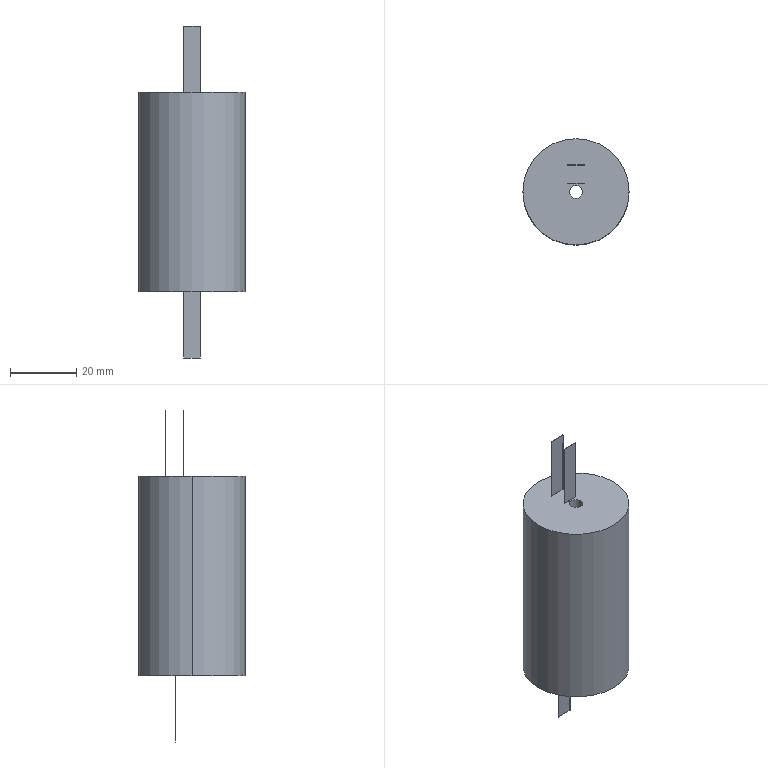Part | SolidWorks | features ICE 2, Extrusion 1 | 1 solid | 21 faces | box 32 x 32 x 100 mm | volume 47531 mm3 | plane 17 | cylinder 4 | commonest cylinder face diameters 4 x2 32 x2
STEP:
#1=CARTESIAN_POINT('',(-2.,0.,60.));
#2=VERTEX_POINT('',#1);
#3=CARTESIAN_POINT('',(2.,0.,60.));
#4=VERTEX_POINT('',#3);
#5=CARTESIAN_POINT('',(0.,0.,60.));
#6=DIRECTION('',(0.,0.,1.));
#7=DIRECTION('',(1.,0.,0.));
#8=AXIS2_PLACEMENT_3D('',#5,#6,#7);
#9=CIRCLE('',#8,2.);
#10=EDGE_CURVE('',#2,#4,#9,.T.);
#11=ORIENTED_EDGE('',*,*,#10,.T.);
#12=CARTESIAN_POINT('',(2.,0.,0.));
#13=VERTEX_POINT('',#12);
#14=CARTESIAN_POINT('',(2.,0.,60.));
#15=DIRECTION('',(0.,0.,-1.));
#16=VECTOR('',#15,1000.);
#17=LINE('',#14,#16);
#18=EDGE_CURVE('',#4,#13,#17,.T.);
#19=ORIENTED_EDGE('',*,*,#18,.T.);
#20=CARTESIAN_POINT('',(-2.,0.,0.));
#21=VERTEX_POINT('',#20);
#22=CARTESIAN_POINT('',(0.,0.,0.));
#23=DIRECTION('',(0.,0.,1.));
#24=DIRECTION('',(1.,0.,0.));
#25=AXIS2_PLACEMENT_3D('',#22,#23,#24);
#26=CIRCLE('',#25,2.);
#27=EDGE_CURVE('',#21,#13,#26,.T.);
#28=ORIENTED_EDGE('',*,*,#27,.F.);
#29=CARTESIAN_POINT('',(-2.,0.,60.));
#30=DIRECTION('',(0.,0.,-1.));
#31=VECTOR('',#30,1000.);
#32=LINE('',#29,#31);
#33=EDGE_CURVE('',#2,#21,#32,.T.);
#34=ORIENTED_EDGE('',*,*,#33,.F.);
#35=EDGE_LOOP('',(#11,#19,#28,#34));
#36=FACE_OUTER_BOUND('',#35,.T.);
#37=CARTESIAN_POINT('',(0.,0.,60.));
#38=DIRECTION('',(0.,0.,-1.));
#39=DIRECTION('',(-1.,0.,0.));
#40=AXIS2_PLACEMENT_3D('',#37,#38,#39);
#41=CYLINDRICAL_SURFACE('',#40,2.);
#42=ADVANCED_FACE('',(#36),#41,.F.);
#43=CARTESIAN_POINT('',(16.,0.,60.));
#44=VERTEX_POINT('',#43);
#45=CARTESIAN_POINT('',(-16.,0.,60.));
#46=VERTEX_POINT('',#45);
#47=CARTESIAN_POINT('',(0.,0.,60.));
#48=DIRECTION('',(0.,0.,1.));
#49=DIRECTION('',(1.,0.,0.));
#50=AXIS2_PLACEMENT_3D('',#47,#48,#49);
#51=CIRCLE('',#50,16.);
#52=EDGE_CURVE('',#44,#46,#51,.T.);
#53=ORIENTED_EDGE('',*,*,#52,.F.);
#54=CARTESIAN_POINT('',(16.,0.,0.));
#55=VERTEX_POINT('',#54);
#56=CARTESIAN_POINT('',(16.,0.,60.));
#57=DIRECTION('',(0.,0.,-1.));
#58=VECTOR('',#57,1000.);
#59=LINE('',#56,#58);
#60=EDGE_CURVE('',#44,#55,#59,.T.);
#61=ORIENTED_EDGE('',*,*,#60,.T.);
#62=CARTESIAN_POINT('',(-16.,0.,0.));
#63=VERTEX_POINT('',#62);
#64=CARTESIAN_POINT('',(0.,0.,0.));
#65=DIRECTION('',(0.,0.,1.));
#66=DIRECTION('',(1.,0.,0.));
#67=AXIS2_PLACEMENT_3D('',#64,#65,#66);
#68=CIRCLE('',#67,16.);
#69=EDGE_CURVE('',#55,#63,#68,.T.);
#70=ORIENTED_EDGE('',*,*,#69,.T.);
#71=CARTESIAN_POINT('',(-16.,0.,60.));
#72=DIRECTION('',(0.,0.,-1.));
#73=VECTOR('',#72,1000.);
#74=LINE('',#71,#73);
#75=EDGE_CURVE('',#46,#63,#74,.T.);
#76=ORIENTED_EDGE('',*,*,#75,.F.);
#77=EDGE_LOOP('',(#53,#61,#70,#76));
#78=FACE_OUTER_BOUND('',#77,.T.);
#79=CARTESIAN_POINT('',(0.,0.,60.));
#80=DIRECTION('',(0.,0.,-1.));
#81=DIRECTION('',(-1.,0.,0.));
#82=AXIS2_PLACEMENT_3D('',#79,#80,#81);
#83=CYLINDRICAL_SURFACE('',#82,16.);
#84=ADVANCED_FACE('',(#78),#83,.T.);
#85=CARTESIAN_POINT('',(2.5,8.1,60.));
#86=VERTEX_POINT('',#85);
#87=CARTESIAN_POINT('',(-2.5,8.1,60.));
#88=VERTEX_POINT('',#87);
#89=CARTESIAN_POINT('',(-2.5,8.1,60.));
#90=DIRECTION('',(-1.,0.,0.));
#91=VECTOR('',#90,1000.);
#92=LINE('',#89,#91);
#93=EDGE_CURVE('',#86,#88,#92,.T.);
#94=ORIENTED_EDGE('',*,*,#93,.F.);
#95=CARTESIAN_POINT('',(2.5,8.,60.));
#96=VERTEX_POINT('',#95);
#97=CARTESIAN_POINT('',(2.5,8.1,60.));
#98=DIRECTION('',(0.,1.,0.));
#99=VECTOR('',#98,1000.);
#100=LINE('',#97,#99);
#101=EDGE_CURVE('',#96,#86,#100,.T.);
#102=ORIENTED_EDGE('',*,*,#101,.F.);
#103=CARTESIAN_POINT('',(-2.5,8.,60.));
#104=VERTEX_POINT('',#103);
#105=CARTESIAN_POINT('',(-2.5,8.,60.));
#106=DIRECTION('',(1.,0.,0.));
#107=VECTOR('',#106,1000.);
#108=LINE('',#105,#107);
#109=EDGE_CURVE('',#104,#96,#108,.T.);
#110=ORIENTED_EDGE('',*,*,#109,.F.);
#111=CARTESIAN_POINT('',(-2.5,8.1,60.));
#112=DIRECTION('',(0.,-1.,0.));
#113=VECTOR('',#112,1000.);
#114=LINE('',#111,#113);
#115=EDGE_CURVE('',#88,#104,#114,.T.);
#116=ORIENTED_EDGE('',*,*,#115,.F.);
#117=EDGE_LOOP('',(#94,#102,#110,#116));
#118=FACE_BOUND('',#117,.T.);
#119=CARTESIAN_POINT('',(0.,0.,60.));
#120=DIRECTION('',(0.,0.,1.));
#121=DIRECTION('',(1.,0.,0.));
#122=AXIS2_PLACEMENT_3D('',#119,#120,#121);
#123=CIRCLE('',#122,16.);
#124=EDGE_CURVE('',#46,#44,#123,.T.);
#125=ORIENTED_EDGE('',*,*,#124,.T.);
#126=ORIENTED_EDGE('',*,*,#52,.T.);
#127=EDGE_LOOP('',(#125,#126));
#128=FACE_OUTER_BOUND('',#127,.T.);
#129=ORIENTED_EDGE('',*,*,#10,.F.);
#130=CARTESIAN_POINT('',(0.,0.,60.));
#131=DIRECTION('',(0.,0.,1.));
#132=DIRECTION('',(1.,0.,0.));
#133=AXIS2_PLACEMENT_3D('',#130,#131,#132);
#134=CIRCLE('',#133,2.);
#135=EDGE_CURVE('',#4,#2,#134,.T.);
#136=ORIENTED_EDGE('',*,*,#135,.F.);
#137=EDGE_LOOP('',(#129,#136));
#138=FACE_BOUND('',#137,.T.);
#139=CARTESIAN_POINT('',(-2.5,2.5,60.));
#140=VERTEX_POINT('',#139);
#141=CARTESIAN_POINT('',(2.5,2.5,60.));
#142=VERTEX_POINT('',#141);
#143=CARTESIAN_POINT('',(-2.5,2.5,60.));
#144=DIRECTION('',(1.,0.,0.));
#145=VECTOR('',#144,1000.);
#146=LINE('',#143,#145);
#147=EDGE_CURVE('',#140,#142,#146,.T.);
#148=ORIENTED_EDGE('',*,*,#147,.F.);
#149=CARTESIAN_POINT('',(-2.5,2.6,60.));
#150=VERTEX_POINT('',#149);
#151=CARTESIAN_POINT('',(-2.5,2.6,60.));
#152=DIRECTION('',(0.,-1.,0.));
#153=VECTOR('',#152,1000.);
#154=LINE('',#151,#153);
#155=EDGE_CURVE('',#150,#140,#154,.T.);
#156=ORIENTED_EDGE('',*,*,#155,.F.);
#157=CARTESIAN_POINT('',(2.5,2.6,60.));
#158=VERTEX_POINT('',#157);
#159=CARTESIAN_POINT('',(-2.5,2.6,60.));
#160=DIRECTION('',(-1.,0.,0.));
#161=VECTOR('',#160,1000.);
#162=LINE('',#159,#161);
#163=EDGE_CURVE('',#158,#150,#162,.T.);
#164=ORIENTED_EDGE('',*,*,#163,.F.);
#165=CARTESIAN_POINT('',(2.5,2.6,60.));
#166=DIRECTION('',(0.,1.,0.));
#167=VECTOR('',#166,1000.);
#168=LINE('',#165,#167);
#169=EDGE_CURVE('',#142,#158,#168,.T.);
#170=ORIENTED_EDGE('',*,*,#169,.F.);
#171=EDGE_LOOP('',(#148,#156,#164,#170));
#172=FACE_BOUND('',#171,.T.);
#173=CARTESIAN_POINT('',(0.,0.,60.));
#174=DIRECTION('',(0.,0.,1.));
#175=DIRECTION('',(1.,0.,0.));
#176=AXIS2_PLACEMENT_3D('',#173,#174,#175);
#177=PLANE('',#176);
#178=ADVANCED_FACE('',(#118,#128,#138,#172),#177,.T.);
#179=ORIENTED_EDGE('',*,*,#27,.T.);
#180=CARTESIAN_POINT('',(0.,0.,0.));
#181=DIRECTION('',(0.,0.,1.));
#182=DIRECTION('',(1.,0.,0.));
#183=AXIS2_PLACEMENT_3D('',#180,#181,#182);
#184=CIRCLE('',#183,2.);
#185=EDGE_CURVE('',#13,#21,#184,.T.);
#186=ORIENTED_EDGE('',*,*,#185,.T.);
#187=EDGE_LOOP('',(#179,#186));
#188=FACE_BOUND('',#187,.T.);
#189=CARTESIAN_POINT('',(0.,0.,0.));
#190=DIRECTION('',(0.,0.,1.));
#191=DIRECTION('',(1.,0.,0.));
#192=AXIS2_PLACEMENT_3D('',#189,#190,#191);
#193=CIRCLE('',#192,16.);
#194=EDGE_CURVE('',#63,#55,#193,.T.);
#195=ORIENTED_EDGE('',*,*,#194,.F.);
#196=ORIENTED_EDGE('',*,*,#69,.F.);
#197=EDGE_LOOP('',(#195,#196));
#198=FACE_OUTER_BOUND('',#197,.T.);
#199=CARTESIAN_POINT('',(-2.5,5.,0.));
#200=VERTEX_POINT('',#199);
#201=CARTESIAN_POINT('',(-2.5,5.1,0.));
#202=VERTEX_POINT('',#201);
#203=CARTESIAN_POINT('',(-2.5,5.1,0.));
#204=DIRECTION('',(0.,1.,0.));
#205=VECTOR('',#204,1000.);
#206=LINE('',#203,#205);
#207=EDGE_CURVE('',#200,#202,#206,.T.);
#208=ORIENTED_EDGE('',*,*,#207,.F.);
#209=CARTESIAN_POINT('',(2.5,5.,0.));
#210=VERTEX_POINT('',#209);
#211=CARTESIAN_POINT('',(2.5,5.,0.));
#212=DIRECTION('',(-1.,0.,0.));
#213=VECTOR('',#212,1000.);
#214=LINE('',#211,#213);
#215=EDGE_CURVE('',#210,#200,#214,.T.);
#216=ORIENTED_EDGE('',*,*,#215,.F.);
#217=CARTESIAN_POINT('',(2.5,5.1,0.));
#218=VERTEX_POINT('',#217);
#219=CARTESIAN_POINT('',(2.5,5.1,0.));
#220=DIRECTION('',(0.,-1.,0.));
#221=VECTOR('',#220,1000.);
#222=LINE('',#219,#221);
#223=EDGE_CURVE('',#218,#210,#222,.T.);
#224=ORIENTED_EDGE('',*,*,#223,.F.);
#225=CARTESIAN_POINT('',(2.5,5.1,0.));
#226=DIRECTION('',(1.,0.,0.));
#227=VECTOR('',#226,1000.);
#228=LINE('',#225,#227);
#229=EDGE_CURVE('',#202,#218,#228,.T.);
#230=ORIENTED_EDGE('',*,*,#229,.F.);
#231=EDGE_LOOP('',(#208,#216,#224,#230));
#232=FACE_BOUND('',#231,.T.);
#233=CARTESIAN_POINT('',(0.,0.,0.));
#234=DIRECTION('',(0.,0.,1.));
#235=DIRECTION('',(1.,0.,0.));
#236=AXIS2_PLACEMENT_3D('',#233,#234,#235);
#237=PLANE('',#236);
#238=ADVANCED_FACE('',(#188,#198,#232),#237,.F.);
#239=ORIENTED_EDGE('',*,*,#60,.F.);
#240=ORIENTED_EDGE('',*,*,#124,.F.);
#241=ORIENTED_EDGE('',*,*,#75,.T.);
#242=ORIENTED_EDGE('',*,*,#194,.T.);
#243=EDGE_LOOP('',(#239,#240,#241,#242));
#244=FACE_OUTER_BOUND('',#243,.T.);
#245=CARTESIAN_POINT('',(0.,0.,60.));
#246=DIRECTION('',(0.,0.,-1.));
#247=DIRECTION('',(-1.,0.,0.));
#248=AXIS2_PLACEMENT_3D('',#245,#246,#247);
#249=CYLINDRICAL_SURFACE('',#248,16.);
#250=ADVANCED_FACE('',(#244),#249,.T.);
#251=ORIENTED_EDGE('',*,*,#18,.F.);
#252=ORIENTED_EDGE('',*,*,#135,.T.);
#253=ORIENTED_EDGE('',*,*,#33,.T.);
#254=ORIENTED_EDGE('',*,*,#185,.F.);
#255=EDGE_LOOP('',(#251,#252,#253,#254));
#256=FACE_OUTER_BOUND('',#255,.T.);
#257=CARTESIAN_POINT('',(0.,0.,60.));
#258=DIRECTION('',(0.,0.,-1.));
#259=DIRECTION('',(-1.,0.,0.));
#260=AXIS2_PLACEMENT_3D('',#257,#258,#259);
#261=CYLINDRICAL_SURFACE('',#260,2.);
#262=ADVANCED_FACE('',(#256),#261,.F.);
#263=ORIENTED_EDGE('',*,*,#207,.T.);
#264=CARTESIAN_POINT('',(-2.5,5.1,-20.));
#265=VERTEX_POINT('',#264);
#266=CARTESIAN_POINT('',(-2.5,5.1,-20.));
#267=DIRECTION('',(0.,0.,1.));
#268=VECTOR('',#267,1000.);
#269=LINE('',#266,#268);
#270=EDGE_CURVE('',#265,#202,#269,.T.);
#271=ORIENTED_EDGE('',*,*,#270,.F.);
#272=CARTESIAN_POINT('',(-2.5,5.,-20.));
#273=VERTEX_POINT('',#272);
#274=CARTESIAN_POINT('',(-2.5,5.1,-20.));
#275=DIRECTION('',(0.,1.,0.));
#276=VECTOR('',#275,1000.);
#277=LINE('',#274,#276);
#278=EDGE_CURVE('',#273,#265,#277,.T.);
#279=ORIENTED_EDGE('',*,*,#278,.F.);
#280=CARTESIAN_POINT('',(-2.5,5.,-20.));
#281=DIRECTION('',(0.,0.,1.));
#282=VECTOR('',#281,1000.);
#283=LINE('',#280,#282);
#284=EDGE_CURVE('',#273,#200,#283,.T.);
#285=ORIENTED_EDGE('',*,*,#284,.T.);
#286=EDGE_LOOP('',(#263,#271,#279,#285));
#287=FACE_OUTER_BOUND('',#286,.T.);
#288=CARTESIAN_POINT('',(-2.5,5.1,-20.));
#289=DIRECTION('',(1.,0.,0.));
#290=DIRECTION('',(0.,0.,-1.));
#291=AXIS2_PLACEMENT_3D('',#288,#289,#290);
#292=PLANE('',#291);
#293=ADVANCED_FACE('',(#287),#292,.F.);
#294=ORIENTED_EDGE('',*,*,#229,.T.);
#295=CARTESIAN_POINT('',(2.5,5.1,-20.));
#296=VERTEX_POINT('',#295);
#297=CARTESIAN_POINT('',(2.5,5.1,-20.));
#298=DIRECTION('',(0.,0.,1.));
#299=VECTOR('',#298,1000.);
#300=LINE('',#297,#299);
#301=EDGE_CURVE('',#296,#218,#300,.T.);
#302=ORIENTED_EDGE('',*,*,#301,.F.);
#303=CARTESIAN_POINT('',(2.5,5.1,-20.));
#304=DIRECTION('',(1.,0.,0.));
#305=VECTOR('',#304,1000.);
#306=LINE('',#303,#305);
#307=EDGE_CURVE('',#265,#296,#306,.T.);
#308=ORIENTED_EDGE('',*,*,#307,.F.);
#309=ORIENTED_EDGE('',*,*,#270,.T.);
#310=EDGE_LOOP('',(#294,#302,#308,#309));
#311=FACE_OUTER_BOUND('',#310,.T.);
#312=CARTESIAN_POINT('',(2.5,5.1,-20.));
#313=DIRECTION('',(0.,-1.,0.));
#314=DIRECTION('',(0.,0.,-1.));
#315=AXIS2_PLACEMENT_3D('',#312,#313,#314);
#316=PLANE('',#315);
#317=ADVANCED_FACE('',(#311),#316,.F.);
#318=ORIENTED_EDGE('',*,*,#223,.T.);
#319=CARTESIAN_POINT('',(2.5,5.,-20.));
#320=VERTEX_POINT('',#319);
#321=CARTESIAN_POINT('',(2.5,5.,-20.));
#322=DIRECTION('',(0.,0.,1.));
#323=VECTOR('',#322,1000.);
#324=LINE('',#321,#323);
#325=EDGE_CURVE('',#320,#210,#324,.T.);
#326=ORIENTED_EDGE('',*,*,#325,.F.);
#327=CARTESIAN_POINT('',(2.5,5.1,-20.));
#328=DIRECTION('',(0.,-1.,0.));
#329=VECTOR('',#328,1000.);
#330=LINE('',#327,#329);
#331=EDGE_CURVE('',#296,#320,#330,.T.);
#332=ORIENTED_EDGE('',*,*,#331,.F.);
#333=ORIENTED_EDGE('',*,*,#301,.T.);
#334=EDGE_LOOP('',(#318,#326,#332,#333));
#335=FACE_OUTER_BOUND('',#334,.T.);
#336=CARTESIAN_POINT('',(2.5,5.1,-20.));
#337=DIRECTION('',(-1.,0.,0.));
#338=DIRECTION('',(0.,0.,1.));
#339=AXIS2_PLACEMENT_3D('',#336,#337,#338);
#340=PLANE('',#339);
#341=ADVANCED_FACE('',(#335),#340,.F.);
#342=ORIENTED_EDGE('',*,*,#215,.T.);
#343=ORIENTED_EDGE('',*,*,#284,.F.);
#344=CARTESIAN_POINT('',(2.5,5.,-20.));
#345=DIRECTION('',(-1.,0.,0.));
#346=VECTOR('',#345,1000.);
#347=LINE('',#344,#346);
#348=EDGE_CURVE('',#320,#273,#347,.T.);
#349=ORIENTED_EDGE('',*,*,#348,.F.);
#350=ORIENTED_EDGE('',*,*,#325,.T.);
#351=EDGE_LOOP('',(#342,#343,#349,#350));
#352=FACE_OUTER_BOUND('',#351,.T.);
#353=CARTESIAN_POINT('',(2.5,5.,-20.));
#354=DIRECTION('',(0.,1.,0.));
#355=DIRECTION('',(0.,0.,1.));
#356=AXIS2_PLACEMENT_3D('',#353,#354,#355);
#357=PLANE('',#356);
#358=ADVANCED_FACE('',(#352),#357,.F.);
#359=ORIENTED_EDGE('',*,*,#278,.T.);
#360=ORIENTED_EDGE('',*,*,#307,.T.);
#361=ORIENTED_EDGE('',*,*,#331,.T.);
#362=ORIENTED_EDGE('',*,*,#348,.T.);
#363=EDGE_LOOP('',(#359,#360,#361,#362));
#364=FACE_OUTER_BOUND('',#363,.T.);
#365=CARTESIAN_POINT('',(0.,0.,-20.));
#366=DIRECTION('',(0.,0.,-1.));
#367=DIRECTION('',(-1.,0.,0.));
#368=AXIS2_PLACEMENT_3D('',#365,#366,#367);
#369=PLANE('',#368);
#370=ADVANCED_FACE('',(#364),#369,.T.);
#371=ORIENTED_EDGE('',*,*,#101,.T.);
#372=CARTESIAN_POINT('',(2.5,8.1,80.));
#373=VERTEX_POINT('',#372);
#374=CARTESIAN_POINT('',(2.5,8.1,80.));
#375=DIRECTION('',(0.,0.,-1.));
#376=VECTOR('',#375,1000.);
#377=LINE('',#374,#376);
#378=EDGE_CURVE('',#373,#86,#377,.T.);
#379=ORIENTED_EDGE('',*,*,#378,.F.);
#380=CARTESIAN_POINT('',(2.5,8.,80.));
#381=VERTEX_POINT('',#380);
#382=CARTESIAN_POINT('',(2.5,8.1,80.));
#383=DIRECTION('',(0.,1.,0.));
#384=VECTOR('',#383,1000.);
#385=LINE('',#382,#384);
#386=EDGE_CURVE('',#381,#373,#385,.T.);
#387=ORIENTED_EDGE('',*,*,#386,.F.);
#388=CARTESIAN_POINT('',(2.5,8.,80.));
#389=DIRECTION('',(0.,0.,-1.));
#390=VECTOR('',#389,1000.);
#391=LINE('',#388,#390);
#392=EDGE_CURVE('',#381,#96,#391,.T.);
#393=ORIENTED_EDGE('',*,*,#392,.T.);
#394=EDGE_LOOP('',(#371,#379,#387,#393));
#395=FACE_OUTER_BOUND('',#394,.T.);
#396=CARTESIAN_POINT('',(2.5,8.1,80.));
#397=DIRECTION('',(-1.,0.,0.));
#398=DIRECTION('',(0.,0.,1.));
#399=AXIS2_PLACEMENT_3D('',#396,#397,#398);
#400=PLANE('',#399);
#401=ADVANCED_FACE('',(#395),#400,.F.);
#402=ORIENTED_EDGE('',*,*,#93,.T.);
#403=CARTESIAN_POINT('',(-2.5,8.1,80.));
#404=VERTEX_POINT('',#403);
#405=CARTESIAN_POINT('',(-2.5,8.1,80.));
#406=DIRECTION('',(0.,0.,-1.));
#407=VECTOR('',#406,1000.);
#408=LINE('',#405,#407);
#409=EDGE_CURVE('',#404,#88,#408,.T.);
#410=ORIENTED_EDGE('',*,*,#409,.F.);
#411=CARTESIAN_POINT('',(-2.5,8.1,80.));
#412=DIRECTION('',(-1.,0.,0.));
#413=VECTOR('',#412,1000.);
#414=LINE('',#411,#413);
#415=EDGE_CURVE('',#373,#404,#414,.T.);
#416=ORIENTED_EDGE('',*,*,#415,.F.);
#417=ORIENTED_EDGE('',*,*,#378,.T.);
#418=EDGE_LOOP('',(#402,#410,#416,#417));
#419=FACE_OUTER_BOUND('',#418,.T.);
#420=CARTESIAN_POINT('',(-2.5,8.1,80.));
#421=DIRECTION('',(0.,-1.,0.));
#422=DIRECTION('',(1.,0.,0.));
#423=AXIS2_PLACEMENT_3D('',#420,#421,#422);
#424=PLANE('',#423);
#425=ADVANCED_FACE('',(#419),#424,.F.);
#426=ORIENTED_EDGE('',*,*,#115,.T.);
#427=CARTESIAN_POINT('',(-2.5,8.,80.));
#428=VERTEX_POINT('',#427);
#429=CARTESIAN_POINT('',(-2.5,8.,80.));
#430=DIRECTION('',(0.,0.,-1.));
#431=VECTOR('',#430,1000.);
#432=LINE('',#429,#431);
#433=EDGE_CURVE('',#428,#104,#432,.T.);
#434=ORIENTED_EDGE('',*,*,#433,.F.);
#435=CARTESIAN_POINT('',(-2.5,8.1,80.));
#436=DIRECTION('',(0.,-1.,0.));
#437=VECTOR('',#436,1000.);
#438=LINE('',#435,#437);
#439=EDGE_CURVE('',#404,#428,#438,.T.);
#440=ORIENTED_EDGE('',*,*,#439,.F.);
#441=ORIENTED_EDGE('',*,*,#409,.T.);
#442=EDGE_LOOP('',(#426,#434,#440,#441));
#443=FACE_OUTER_BOUND('',#442,.T.);
#444=CARTESIAN_POINT('',(-2.5,8.1,80.));
#445=DIRECTION('',(1.,0.,0.));
#446=DIRECTION('',(0.,0.,-1.));
#447=AXIS2_PLACEMENT_3D('',#444,#445,#446);
#448=PLANE('',#447);
#449=ADVANCED_FACE('',(#443),#448,.F.);
#450=ORIENTED_EDGE('',*,*,#109,.T.);
#451=ORIENTED_EDGE('',*,*,#392,.F.);
#452=CARTESIAN_POINT('',(-2.5,8.,80.));
#453=DIRECTION('',(1.,0.,0.));
#454=VECTOR('',#453,1000.);
#455=LINE('',#452,#454);
#456=EDGE_CURVE('',#428,#381,#455,.T.);
#457=ORIENTED_EDGE('',*,*,#456,.F.);
#458=ORIENTED_EDGE('',*,*,#433,.T.);
#459=EDGE_LOOP('',(#450,#451,#457,#458));
#460=FACE_OUTER_BOUND('',#459,.T.);
#461=CARTESIAN_POINT('',(-2.5,8.,80.));
#462=DIRECTION('',(0.,1.,0.));
#463=DIRECTION('',(0.,0.,1.));
#464=AXIS2_PLACEMENT_3D('',#461,#462,#463);
#465=PLANE('',#464);
#466=ADVANCED_FACE('',(#460),#465,.F.);
#467=ORIENTED_EDGE('',*,*,#386,.T.);
#468=ORIENTED_EDGE('',*,*,#415,.T.);
#469=ORIENTED_EDGE('',*,*,#439,.T.);
#470=ORIENTED_EDGE('',*,*,#456,.T.);
#471=EDGE_LOOP('',(#467,#468,#469,#470));
#472=FACE_OUTER_BOUND('',#471,.T.);
#473=CARTESIAN_POINT('',(0.,0.,80.));
#474=DIRECTION('',(0.,0.,1.));
#475=DIRECTION('',(1.,0.,0.));
#476=AXIS2_PLACEMENT_3D('',#473,#474,#475);
#477=PLANE('',#476);
#478=ADVANCED_FACE('',(#472),#477,.T.);
#479=ORIENTED_EDGE('',*,*,#155,.T.);
#480=CARTESIAN_POINT('',(-2.5,2.5,80.));
#481=VERTEX_POINT('',#480);
#482=CARTESIAN_POINT('',(-2.5,2.5,80.));
#483=DIRECTION('',(0.,0.,-1.));
#484=VECTOR('',#483,1000.);
#485=LINE('',#482,#484);
#486=EDGE_CURVE('',#481,#140,#485,.T.);
#487=ORIENTED_EDGE('',*,*,#486,.F.);
#488=CARTESIAN_POINT('',(-2.5,2.6,80.));
#489=VERTEX_POINT('',#488);
#490=CARTESIAN_POINT('',(-2.5,2.6,80.));
#491=DIRECTION('',(0.,-1.,0.));
#492=VECTOR('',#491,1000.);
#493=LINE('',#490,#492);
#494=EDGE_CURVE('',#489,#481,#493,.T.);
#495=ORIENTED_EDGE('',*,*,#494,.F.);
#496=CARTESIAN_POINT('',(-2.5,2.6,80.));
#497=DIRECTION('',(0.,0.,-1.));
#498=VECTOR('',#497,1000.);
#499=LINE('',#496,#498);
#500=EDGE_CURVE('',#489,#150,#499,.T.);
#501=ORIENTED_EDGE('',*,*,#500,.T.);
#502=EDGE_LOOP('',(#479,#487,#495,#501));
#503=FACE_OUTER_BOUND('',#502,.T.);
#504=CARTESIAN_POINT('',(-2.5,2.6,80.));
#505=DIRECTION('',(1.,0.,0.));
#506=DIRECTION('',(0.,1.,0.));
#507=AXIS2_PLACEMENT_3D('',#504,#505,#506);
#508=PLANE('',#507);
#509=ADVANCED_FACE('',(#503),#508,.F.);
#510=ORIENTED_EDGE('',*,*,#147,.T.);
#511=CARTESIAN_POINT('',(2.5,2.5,80.));
#512=VERTEX_POINT('',#511);
#513=CARTESIAN_POINT('',(2.5,2.5,80.));
#514=DIRECTION('',(0.,0.,-1.));
#515=VECTOR('',#514,1000.);
#516=LINE('',#513,#515);
#517=EDGE_CURVE('',#512,#142,#516,.T.);
#518=ORIENTED_EDGE('',*,*,#517,.F.);
#519=CARTESIAN_POINT('',(-2.5,2.5,80.));
#520=DIRECTION('',(1.,0.,0.));
#521=VECTOR('',#520,1000.);
#522=LINE('',#519,#521);
#523=EDGE_CURVE('',#481,#512,#522,.T.);
#524=ORIENTED_EDGE('',*,*,#523,.F.);
#525=ORIENTED_EDGE('',*,*,#486,.T.);
#526=EDGE_LOOP('',(#510,#518,#524,#525));
#527=FACE_OUTER_BOUND('',#526,.T.);
#528=CARTESIAN_POINT('',(-2.5,2.5,80.));
#529=DIRECTION('',(0.,1.,0.));
#530=DIRECTION('',(0.,0.,1.));
#531=AXIS2_PLACEMENT_3D('',#528,#529,#530);
#532=PLANE('',#531);
#533=ADVANCED_FACE('',(#527),#532,.F.);
#534=ORIENTED_EDGE('',*,*,#169,.T.);
#535=CARTESIAN_POINT('',(2.5,2.6,80.));
#536=VERTEX_POINT('',#535);
#537=CARTESIAN_POINT('',(2.5,2.6,80.));
#538=DIRECTION('',(0.,0.,-1.));
#539=VECTOR('',#538,1000.);
#540=LINE('',#537,#539);
#541=EDGE_CURVE('',#536,#158,#540,.T.);
#542=ORIENTED_EDGE('',*,*,#541,.F.);
#543=CARTESIAN_POINT('',(2.5,2.6,80.));
#544=DIRECTION('',(0.,1.,0.));
#545=VECTOR('',#544,1000.);
#546=LINE('',#543,#545);
#547=EDGE_CURVE('',#512,#536,#546,.T.);
#548=ORIENTED_EDGE('',*,*,#547,.F.);
#549=ORIENTED_EDGE('',*,*,#517,.T.);
#550=EDGE_LOOP('',(#534,#542,#548,#549));
#551=FACE_OUTER_BOUND('',#550,.T.);
#552=CARTESIAN_POINT('',(2.5,2.6,80.));
#553=DIRECTION('',(-1.,0.,0.));
#554=DIRECTION('',(0.,-1.,0.));
#555=AXIS2_PLACEMENT_3D('',#552,#553,#554);
#556=PLANE('',#555);
#557=ADVANCED_FACE('',(#551),#556,.F.);
#558=ORIENTED_EDGE('',*,*,#163,.T.);
#559=ORIENTED_EDGE('',*,*,#500,.F.);
#560=CARTESIAN_POINT('',(-2.5,2.6,80.));
#561=DIRECTION('',(-1.,0.,0.));
#562=VECTOR('',#561,1000.);
#563=LINE('',#560,#562);
#564=EDGE_CURVE('',#536,#489,#563,.T.);
#565=ORIENTED_EDGE('',*,*,#564,.F.);
#566=ORIENTED_EDGE('',*,*,#541,.T.);
#567=EDGE_LOOP('',(#558,#559,#565,#566));
#568=FACE_OUTER_BOUND('',#567,.T.);
#569=CARTESIAN_POINT('',(-2.5,2.6,80.));
#570=DIRECTION('',(0.,-1.,0.));
#571=DIRECTION('',(0.,0.,-1.));
#572=AXIS2_PLACEMENT_3D('',#569,#570,#571);
#573=PLANE('',#572);
#574=ADVANCED_FACE('',(#568),#573,.F.);
#575=ORIENTED_EDGE('',*,*,#494,.T.);
#576=ORIENTED_EDGE('',*,*,#523,.T.);
#577=ORIENTED_EDGE('',*,*,#547,.T.);
#578=ORIENTED_EDGE('',*,*,#564,.T.);
#579=EDGE_LOOP('',(#575,#576,#577,#578));
#580=FACE_OUTER_BOUND('',#579,.T.);
#581=CARTESIAN_POINT('',(0.,0.,80.));
#582=DIRECTION('',(0.,0.,1.));
#583=DIRECTION('',(1.,0.,0.));
#584=AXIS2_PLACEMENT_3D('',#581,#582,#583);
#585=PLANE('',#584);
#586=ADVANCED_FACE('',(#580),#585,.T.);
#587=CLOSED_SHELL('',(#42,#84,#178,#238,#250,#262,#293,#317,#341,#358,#370,#401,#425,#449,#466,#478,#509,#533,#557,#574,#586));
#588=MANIFOLD_SOLID_BREP('',#587);
#589=CARTESIAN_POINT('',(0.,0.,0.));
#590=DIRECTION('',(0.,0.,1.));
#591=DIRECTION('',(1.,0.,0.));
#592=AXIS2_PLACEMENT_3D('',#589,#590,#591);
#593=(LENGTH_UNIT()NAMED_UNIT(*)SI_UNIT(.MILLI.,.METRE.));
#594=UNCERTAINTY_MEASURE_WITH_UNIT(LENGTH_MEASURE(0.00001),#593,'','');
#595=(NAMED_UNIT(*)PLANE_ANGLE_UNIT()SI_UNIT($,.RADIAN.));
#596=(NAMED_UNIT(*)SI_UNIT($,.STERADIAN.)SOLID_ANGLE_UNIT());
#597=(GEOMETRIC_REPRESENTATION_CONTEXT(3)GLOBAL_UNCERTAINTY_ASSIGNED_CONTEXT((#594))GLOBAL_UNIT_ASSIGNED_CONTEXT((#593,#595,#596))REPRESENTATION_CONTEXT('',''));
#598=ADVANCED_BREP_SHAPE_REPRESENTATION('',(#588,#592),#597);